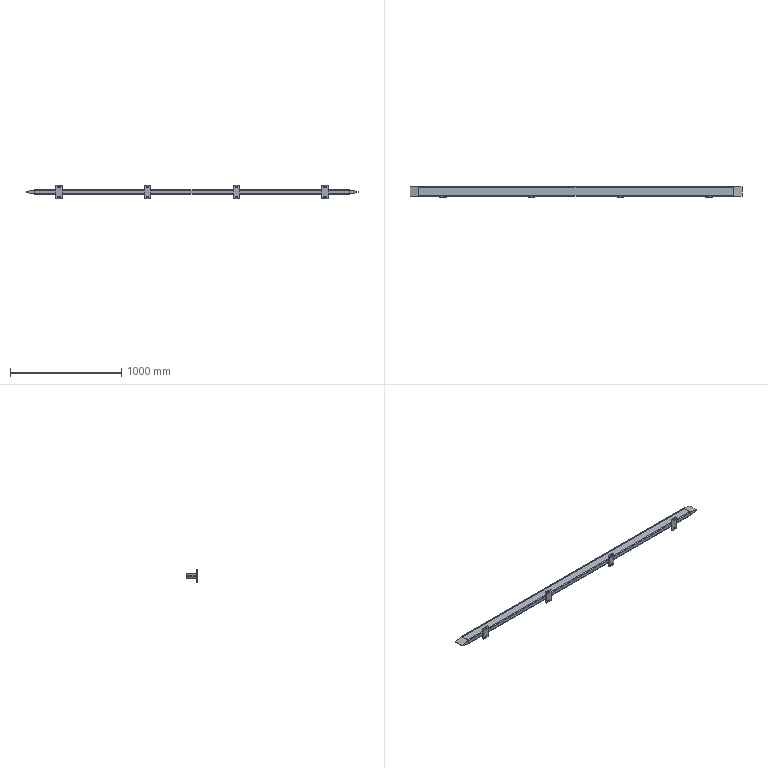Part | SolidWorks | features ICE 5, MirrorSolid 2, HoleWzd 1, WeldMemberFeat 1, WeldmentFeature 1 | 10 solids | 276 faces | box 2990 x 95 x 120 mm | volume 3021491 mm3 | cylinder 180 | plane 96 | commonest cylinder face diameters 6.8 x148 13.5 x16 6 x12 12 x4